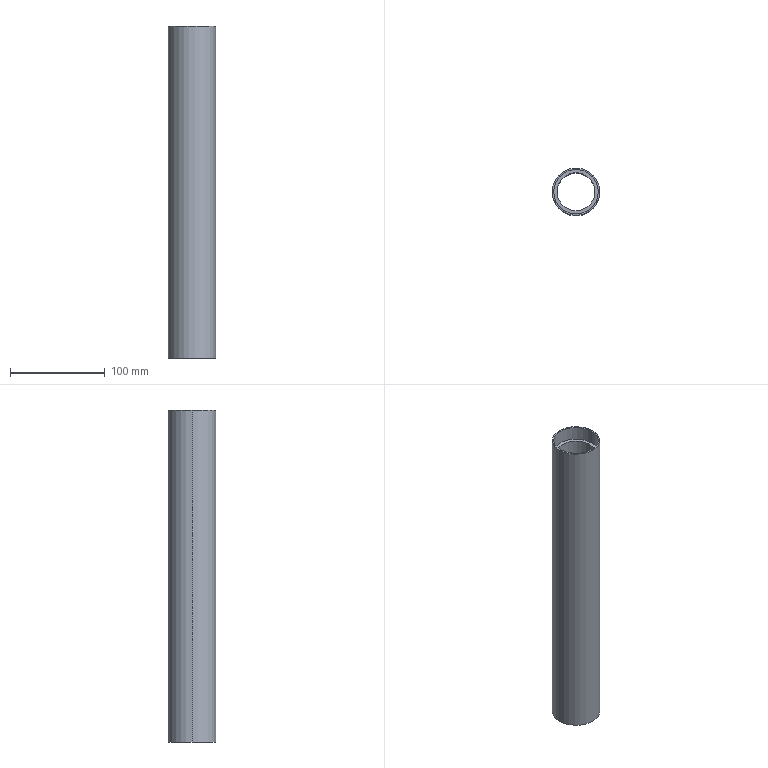Part | STEP file | Roller 2 | 1 solid | 12 faces | box 50 x 50 x 350 mm | volume 233051 mm3 | cylinder 8 | plane 4 | commonest cylinder face diameters 47 x4 40 x2 50 x2
STEP:
#1=CARTESIAN_POINT('',(-25.,0.,350.));
#2=VERTEX_POINT('',#1);
#3=CARTESIAN_POINT('',(25.,0.,350.));
#4=VERTEX_POINT('',#3);
#5=CARTESIAN_POINT('',(0.,0.,350.));
#6=DIRECTION('',(0.,0.,-1.));
#7=DIRECTION('',(-1.,0.,0.));
#8=AXIS2_PLACEMENT_3D('',#5,#6,#7);
#9=CIRCLE('',#8,25.);
#10=EDGE_CURVE('',#2,#4,#9,.T.);
#11=ORIENTED_EDGE('',*,*,#10,.T.);
#12=CARTESIAN_POINT('',(25.,0.,0.));
#13=VERTEX_POINT('',#12);
#14=CARTESIAN_POINT('',(25.,0.,350.));
#15=DIRECTION('',(0.,0.,-1.));
#16=VECTOR('',#15,1000.);
#17=LINE('',#14,#16);
#18=EDGE_CURVE('',#4,#13,#17,.T.);
#19=ORIENTED_EDGE('',*,*,#18,.T.);
#20=CARTESIAN_POINT('',(-25.,0.,0.));
#21=VERTEX_POINT('',#20);
#22=CARTESIAN_POINT('',(0.,0.,0.));
#23=DIRECTION('',(0.,0.,1.));
#24=DIRECTION('',(-1.,0.,0.));
#25=AXIS2_PLACEMENT_3D('',#22,#23,#24);
#26=CIRCLE('',#25,25.);
#27=EDGE_CURVE('',#13,#21,#26,.T.);
#28=ORIENTED_EDGE('',*,*,#27,.T.);
#29=CARTESIAN_POINT('',(-25.,0.,350.));
#30=DIRECTION('',(0.,0.,-1.));
#31=VECTOR('',#30,1000.);
#32=LINE('',#29,#31);
#33=EDGE_CURVE('',#2,#21,#32,.T.);
#34=ORIENTED_EDGE('',*,*,#33,.F.);
#35=EDGE_LOOP('',(#11,#19,#28,#34));
#36=FACE_OUTER_BOUND('',#35,.T.);
#37=CARTESIAN_POINT('',(0.,0.,350.));
#38=DIRECTION('',(0.,0.,-1.));
#39=DIRECTION('',(-1.,0.,0.));
#40=AXIS2_PLACEMENT_3D('',#37,#38,#39);
#41=CYLINDRICAL_SURFACE('',#40,25.);
#42=ADVANCED_FACE('',(#36),#41,.T.);
#43=CARTESIAN_POINT('',(23.5,0.,15.));
#44=VERTEX_POINT('',#43);
#45=CARTESIAN_POINT('',(-23.5,0.,15.));
#46=VERTEX_POINT('',#45);
#47=CARTESIAN_POINT('',(0.,0.,15.));
#48=DIRECTION('',(0.,0.,-1.));
#49=DIRECTION('',(-1.,0.,0.));
#50=AXIS2_PLACEMENT_3D('',#47,#48,#49);
#51=CIRCLE('',#50,23.5);
#52=EDGE_CURVE('',#44,#46,#51,.T.);
#53=ORIENTED_EDGE('',*,*,#52,.F.);
#54=CARTESIAN_POINT('',(23.5,0.,0.));
#55=VERTEX_POINT('',#54);
#56=CARTESIAN_POINT('',(23.5,0.,15.));
#57=DIRECTION('',(0.,0.,-1.));
#58=VECTOR('',#57,1000.);
#59=LINE('',#56,#58);
#60=EDGE_CURVE('',#44,#55,#59,.T.);
#61=ORIENTED_EDGE('',*,*,#60,.T.);
#62=CARTESIAN_POINT('',(-23.5,0.,0.));
#63=VERTEX_POINT('',#62);
#64=CARTESIAN_POINT('',(0.,0.,0.));
#65=DIRECTION('',(0.,0.,-1.));
#66=DIRECTION('',(-1.,0.,0.));
#67=AXIS2_PLACEMENT_3D('',#64,#65,#66);
#68=CIRCLE('',#67,23.5);
#69=EDGE_CURVE('',#55,#63,#68,.T.);
#70=ORIENTED_EDGE('',*,*,#69,.T.);
#71=CARTESIAN_POINT('',(-23.5,0.,15.));
#72=DIRECTION('',(0.,0.,-1.));
#73=VECTOR('',#72,1000.);
#74=LINE('',#71,#73);
#75=EDGE_CURVE('',#46,#63,#74,.T.);
#76=ORIENTED_EDGE('',*,*,#75,.F.);
#77=EDGE_LOOP('',(#53,#61,#70,#76));
#78=FACE_OUTER_BOUND('',#77,.T.);
#79=CARTESIAN_POINT('',(0.,0.,15.));
#80=DIRECTION('',(0.,0.,-1.));
#81=DIRECTION('',(-1.,0.,0.));
#82=AXIS2_PLACEMENT_3D('',#79,#80,#81);
#83=CYLINDRICAL_SURFACE('',#82,23.5);
#84=ADVANCED_FACE('',(#78),#83,.F.);
#85=CARTESIAN_POINT('',(-23.5,0.,335.));
#86=VERTEX_POINT('',#85);
#87=CARTESIAN_POINT('',(23.5,0.,335.));
#88=VERTEX_POINT('',#87);
#89=CARTESIAN_POINT('',(0.,0.,335.));
#90=DIRECTION('',(0.,0.,1.));
#91=DIRECTION('',(1.,0.,0.));
#92=AXIS2_PLACEMENT_3D('',#89,#90,#91);
#93=CIRCLE('',#92,23.5);
#94=EDGE_CURVE('',#86,#88,#93,.T.);
#95=ORIENTED_EDGE('',*,*,#94,.F.);
#96=CARTESIAN_POINT('',(-23.5,0.,350.));
#97=VERTEX_POINT('',#96);
#98=CARTESIAN_POINT('',(-23.5,0.,335.));
#99=DIRECTION('',(0.,0.,1.));
#100=VECTOR('',#99,1000.);
#101=LINE('',#98,#100);
#102=EDGE_CURVE('',#86,#97,#101,.T.);
#103=ORIENTED_EDGE('',*,*,#102,.T.);
#104=CARTESIAN_POINT('',(23.5,0.,350.));
#105=VERTEX_POINT('',#104);
#106=CARTESIAN_POINT('',(0.,0.,350.));
#107=DIRECTION('',(0.,0.,-1.));
#108=DIRECTION('',(1.,0.,0.));
#109=AXIS2_PLACEMENT_3D('',#106,#107,#108);
#110=CIRCLE('',#109,23.5);
#111=EDGE_CURVE('',#105,#97,#110,.T.);
#112=ORIENTED_EDGE('',*,*,#111,.F.);
#113=CARTESIAN_POINT('',(23.5,0.,335.));
#114=DIRECTION('',(0.,0.,1.));
#115=VECTOR('',#114,1000.);
#116=LINE('',#113,#115);
#117=EDGE_CURVE('',#88,#105,#116,.T.);
#118=ORIENTED_EDGE('',*,*,#117,.F.);
#119=EDGE_LOOP('',(#95,#103,#112,#118));
#120=FACE_OUTER_BOUND('',#119,.T.);
#121=CARTESIAN_POINT('',(0.,0.,335.));
#122=DIRECTION('',(0.,0.,1.));
#123=DIRECTION('',(1.,0.,0.));
#124=AXIS2_PLACEMENT_3D('',#121,#122,#123);
#125=CYLINDRICAL_SURFACE('',#124,23.5);
#126=ADVANCED_FACE('',(#120),#125,.F.);
#127=CARTESIAN_POINT('',(20.,0.,335.));
#128=VERTEX_POINT('',#127);
#129=CARTESIAN_POINT('',(-20.,0.,335.));
#130=VERTEX_POINT('',#129);
#131=CARTESIAN_POINT('',(0.,0.,335.));
#132=DIRECTION('',(0.,0.,-1.));
#133=DIRECTION('',(-1.,0.,0.));
#134=AXIS2_PLACEMENT_3D('',#131,#132,#133);
#135=CIRCLE('',#134,20.);
#136=EDGE_CURVE('',#128,#130,#135,.T.);
#137=ORIENTED_EDGE('',*,*,#136,.F.);
#138=CARTESIAN_POINT('',(20.,0.,15.));
#139=VERTEX_POINT('',#138);
#140=CARTESIAN_POINT('',(20.,0.,350.));
#141=DIRECTION('',(0.,0.,-1.));
#142=VECTOR('',#141,1000.);
#143=LINE('',#140,#142);
#144=EDGE_CURVE('',#128,#139,#143,.T.);
#145=ORIENTED_EDGE('',*,*,#144,.T.);
#146=CARTESIAN_POINT('',(-20.,0.,15.));
#147=VERTEX_POINT('',#146);
#148=CARTESIAN_POINT('',(0.,0.,15.));
#149=DIRECTION('',(0.,0.,1.));
#150=DIRECTION('',(-1.,0.,0.));
#151=AXIS2_PLACEMENT_3D('',#148,#149,#150);
#152=CIRCLE('',#151,20.);
#153=EDGE_CURVE('',#147,#139,#152,.T.);
#154=ORIENTED_EDGE('',*,*,#153,.F.);
#155=CARTESIAN_POINT('',(-20.,0.,350.));
#156=DIRECTION('',(0.,0.,-1.));
#157=VECTOR('',#156,1000.);
#158=LINE('',#155,#157);
#159=EDGE_CURVE('',#130,#147,#158,.T.);
#160=ORIENTED_EDGE('',*,*,#159,.F.);
#161=EDGE_LOOP('',(#137,#145,#154,#160));
#162=FACE_OUTER_BOUND('',#161,.T.);
#163=CARTESIAN_POINT('',(0.,0.,350.));
#164=DIRECTION('',(0.,0.,-1.));
#165=DIRECTION('',(-1.,0.,0.));
#166=AXIS2_PLACEMENT_3D('',#163,#164,#165);
#167=CYLINDRICAL_SURFACE('',#166,20.);
#168=ADVANCED_FACE('',(#162),#167,.F.);
#169=ORIENTED_EDGE('',*,*,#18,.F.);
#170=CARTESIAN_POINT('',(0.,0.,350.));
#171=DIRECTION('',(0.,0.,-1.));
#172=DIRECTION('',(-1.,0.,0.));
#173=AXIS2_PLACEMENT_3D('',#170,#171,#172);
#174=CIRCLE('',#173,25.);
#175=EDGE_CURVE('',#4,#2,#174,.T.);
#176=ORIENTED_EDGE('',*,*,#175,.T.);
#177=ORIENTED_EDGE('',*,*,#33,.T.);
#178=CARTESIAN_POINT('',(0.,0.,0.));
#179=DIRECTION('',(0.,0.,1.));
#180=DIRECTION('',(-1.,0.,0.));
#181=AXIS2_PLACEMENT_3D('',#178,#179,#180);
#182=CIRCLE('',#181,25.);
#183=EDGE_CURVE('',#21,#13,#182,.T.);
#184=ORIENTED_EDGE('',*,*,#183,.T.);
#185=EDGE_LOOP('',(#169,#176,#177,#184));
#186=FACE_OUTER_BOUND('',#185,.T.);
#187=CARTESIAN_POINT('',(0.,0.,350.));
#188=DIRECTION('',(0.,0.,-1.));
#189=DIRECTION('',(-1.,0.,0.));
#190=AXIS2_PLACEMENT_3D('',#187,#188,#189);
#191=CYLINDRICAL_SURFACE('',#190,25.);
#192=ADVANCED_FACE('',(#186),#191,.T.);
#193=ORIENTED_EDGE('',*,*,#183,.F.);
#194=ORIENTED_EDGE('',*,*,#27,.F.);
#195=EDGE_LOOP('',(#193,#194));
#196=FACE_OUTER_BOUND('',#195,.T.);
#197=CARTESIAN_POINT('',(0.,0.,0.));
#198=DIRECTION('',(0.,0.,-1.));
#199=DIRECTION('',(-1.,0.,0.));
#200=AXIS2_PLACEMENT_3D('',#197,#198,#199);
#201=CIRCLE('',#200,23.5);
#202=EDGE_CURVE('',#63,#55,#201,.T.);
#203=ORIENTED_EDGE('',*,*,#202,.F.);
#204=ORIENTED_EDGE('',*,*,#69,.F.);
#205=EDGE_LOOP('',(#203,#204));
#206=FACE_BOUND('',#205,.T.);
#207=CARTESIAN_POINT('',(0.,0.,0.));
#208=DIRECTION('',(0.,0.,1.));
#209=DIRECTION('',(1.,0.,0.));
#210=AXIS2_PLACEMENT_3D('',#207,#208,#209);
#211=PLANE('',#210);
#212=ADVANCED_FACE('',(#196,#206),#211,.F.);
#213=ORIENTED_EDGE('',*,*,#10,.F.);
#214=ORIENTED_EDGE('',*,*,#175,.F.);
#215=EDGE_LOOP('',(#213,#214));
#216=FACE_OUTER_BOUND('',#215,.T.);
#217=ORIENTED_EDGE('',*,*,#111,.T.);
#218=CARTESIAN_POINT('',(0.,0.,350.));
#219=DIRECTION('',(0.,0.,-1.));
#220=DIRECTION('',(1.,0.,0.));
#221=AXIS2_PLACEMENT_3D('',#218,#219,#220);
#222=CIRCLE('',#221,23.5);
#223=EDGE_CURVE('',#97,#105,#222,.T.);
#224=ORIENTED_EDGE('',*,*,#223,.T.);
#225=EDGE_LOOP('',(#217,#224));
#226=FACE_BOUND('',#225,.T.);
#227=CARTESIAN_POINT('',(0.,0.,350.));
#228=DIRECTION('',(0.,0.,1.));
#229=DIRECTION('',(1.,0.,0.));
#230=AXIS2_PLACEMENT_3D('',#227,#228,#229);
#231=PLANE('',#230);
#232=ADVANCED_FACE('',(#216,#226),#231,.T.);
#233=ORIENTED_EDGE('',*,*,#60,.F.);
#234=CARTESIAN_POINT('',(0.,0.,15.));
#235=DIRECTION('',(0.,0.,-1.));
#236=DIRECTION('',(-1.,0.,0.));
#237=AXIS2_PLACEMENT_3D('',#234,#235,#236);
#238=CIRCLE('',#237,23.5);
#239=EDGE_CURVE('',#46,#44,#238,.T.);
#240=ORIENTED_EDGE('',*,*,#239,.F.);
#241=ORIENTED_EDGE('',*,*,#75,.T.);
#242=ORIENTED_EDGE('',*,*,#202,.T.);
#243=EDGE_LOOP('',(#233,#240,#241,#242));
#244=FACE_OUTER_BOUND('',#243,.T.);
#245=CARTESIAN_POINT('',(0.,0.,15.));
#246=DIRECTION('',(0.,0.,-1.));
#247=DIRECTION('',(-1.,0.,0.));
#248=AXIS2_PLACEMENT_3D('',#245,#246,#247);
#249=CYLINDRICAL_SURFACE('',#248,23.5);
#250=ADVANCED_FACE('',(#244),#249,.F.);
#251=ORIENTED_EDGE('',*,*,#102,.F.);
#252=CARTESIAN_POINT('',(0.,0.,335.));
#253=DIRECTION('',(0.,0.,1.));
#254=DIRECTION('',(1.,0.,0.));
#255=AXIS2_PLACEMENT_3D('',#252,#253,#254);
#256=CIRCLE('',#255,23.5);
#257=EDGE_CURVE('',#88,#86,#256,.T.);
#258=ORIENTED_EDGE('',*,*,#257,.F.);
#259=ORIENTED_EDGE('',*,*,#117,.T.);
#260=ORIENTED_EDGE('',*,*,#223,.F.);
#261=EDGE_LOOP('',(#251,#258,#259,#260));
#262=FACE_OUTER_BOUND('',#261,.T.);
#263=CARTESIAN_POINT('',(0.,0.,335.));
#264=DIRECTION('',(0.,0.,1.));
#265=DIRECTION('',(1.,0.,0.));
#266=AXIS2_PLACEMENT_3D('',#263,#264,#265);
#267=CYLINDRICAL_SURFACE('',#266,23.5);
#268=ADVANCED_FACE('',(#262),#267,.F.);
#269=ORIENTED_EDGE('',*,*,#239,.T.);
#270=ORIENTED_EDGE('',*,*,#52,.T.);
#271=EDGE_LOOP('',(#269,#270));
#272=FACE_OUTER_BOUND('',#271,.T.);
#273=ORIENTED_EDGE('',*,*,#153,.T.);
#274=CARTESIAN_POINT('',(0.,0.,15.));
#275=DIRECTION('',(0.,0.,1.));
#276=DIRECTION('',(-1.,0.,0.));
#277=AXIS2_PLACEMENT_3D('',#274,#275,#276);
#278=CIRCLE('',#277,20.);
#279=EDGE_CURVE('',#139,#147,#278,.T.);
#280=ORIENTED_EDGE('',*,*,#279,.T.);
#281=EDGE_LOOP('',(#273,#280));
#282=FACE_BOUND('',#281,.T.);
#283=CARTESIAN_POINT('',(0.,0.,15.));
#284=DIRECTION('',(0.,0.,-1.));
#285=DIRECTION('',(-1.,0.,0.));
#286=AXIS2_PLACEMENT_3D('',#283,#284,#285);
#287=PLANE('',#286);
#288=ADVANCED_FACE('',(#272,#282),#287,.T.);
#289=ORIENTED_EDGE('',*,*,#257,.T.);
#290=ORIENTED_EDGE('',*,*,#94,.T.);
#291=EDGE_LOOP('',(#289,#290));
#292=FACE_OUTER_BOUND('',#291,.T.);
#293=CARTESIAN_POINT('',(0.,0.,335.));
#294=DIRECTION('',(0.,0.,-1.));
#295=DIRECTION('',(-1.,0.,0.));
#296=AXIS2_PLACEMENT_3D('',#293,#294,#295);
#297=CIRCLE('',#296,20.);
#298=EDGE_CURVE('',#130,#128,#297,.T.);
#299=ORIENTED_EDGE('',*,*,#298,.T.);
#300=ORIENTED_EDGE('',*,*,#136,.T.);
#301=EDGE_LOOP('',(#299,#300));
#302=FACE_BOUND('',#301,.T.);
#303=CARTESIAN_POINT('',(0.,0.,335.));
#304=DIRECTION('',(0.,0.,1.));
#305=DIRECTION('',(1.,0.,0.));
#306=AXIS2_PLACEMENT_3D('',#303,#304,#305);
#307=PLANE('',#306);
#308=ADVANCED_FACE('',(#292,#302),#307,.T.);
#309=ORIENTED_EDGE('',*,*,#144,.F.);
#310=ORIENTED_EDGE('',*,*,#298,.F.);
#311=ORIENTED_EDGE('',*,*,#159,.T.);
#312=ORIENTED_EDGE('',*,*,#279,.F.);
#313=EDGE_LOOP('',(#309,#310,#311,#312));
#314=FACE_OUTER_BOUND('',#313,.T.);
#315=CARTESIAN_POINT('',(0.,0.,350.));
#316=DIRECTION('',(0.,0.,-1.));
#317=DIRECTION('',(-1.,0.,0.));
#318=AXIS2_PLACEMENT_3D('',#315,#316,#317);
#319=CYLINDRICAL_SURFACE('',#318,20.);
#320=ADVANCED_FACE('',(#314),#319,.F.);
#321=CLOSED_SHELL('',(#42,#84,#126,#168,#192,#212,#232,#250,#268,#288,#308,#320));
#322=MANIFOLD_SOLID_BREP('',#321);
#323=CARTESIAN_POINT('',(0.,0.,0.));
#324=DIRECTION('',(0.,0.,1.));
#325=DIRECTION('',(1.,0.,0.));
#326=AXIS2_PLACEMENT_3D('',#323,#324,#325);
#327=(LENGTH_UNIT()NAMED_UNIT(*)SI_UNIT(.MILLI.,.METRE.));
#328=UNCERTAINTY_MEASURE_WITH_UNIT(LENGTH_MEASURE(0.00001),#327,'','');
#329=(NAMED_UNIT(*)PLANE_ANGLE_UNIT()SI_UNIT($,.RADIAN.));
#330=(NAMED_UNIT(*)SI_UNIT($,.STERADIAN.)SOLID_ANGLE_UNIT());
#331=(GEOMETRIC_REPRESENTATION_CONTEXT(3)GLOBAL_UNCERTAINTY_ASSIGNED_CONTEXT((#328))GLOBAL_UNIT_ASSIGNED_CONTEXT((#327,#329,#330))REPRESENTATION_CONTEXT('',''));
#332=ADVANCED_BREP_SHAPE_REPRESENTATION('',(#322,#326),#331);